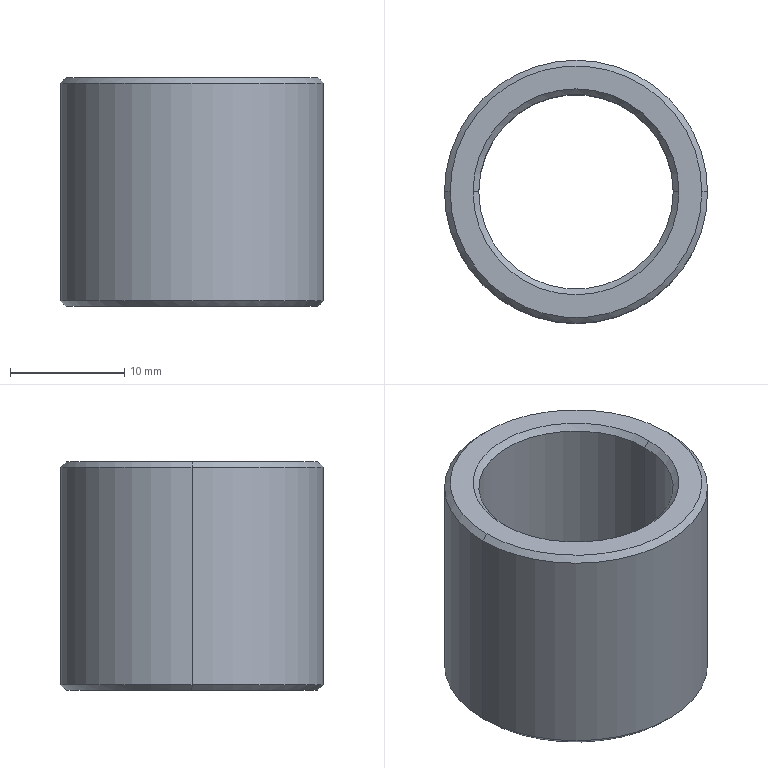Part | SolidWorks | features Chamfer 1, Extrusion 1 | 1 solid | 14 faces | box 23 x 23 x 20 mm | volume 3738 mm3 | cone 8 | cylinder 4 | plane 2 | commonest cylinder face diameters 17 x2 23 x2
STEP:
#1=CARTESIAN_POINT('',(-8.5,0.,19.5));
#2=VERTEX_POINT('',#1);
#3=CARTESIAN_POINT('',(8.5,0.,19.5));
#4=VERTEX_POINT('',#3);
#5=CARTESIAN_POINT('',(0.,0.,19.5));
#6=DIRECTION('',(0.,0.,1.));
#7=DIRECTION('',(1.,0.,0.));
#8=AXIS2_PLACEMENT_3D('',#5,#6,#7);
#9=CIRCLE('',#8,8.5);
#10=EDGE_CURVE('',#2,#4,#9,.T.);
#11=ORIENTED_EDGE('',*,*,#10,.F.);
#12=CARTESIAN_POINT('',(-9.,0.,20.));
#13=VERTEX_POINT('',#12);
#14=CARTESIAN_POINT('',(-8.5,0.,19.5));
#15=DIRECTION('',(-0.7071,0.,0.7071));
#16=VECTOR('',#15,1000.);
#17=LINE('',#14,#16);
#18=EDGE_CURVE('',#2,#13,#17,.T.);
#19=ORIENTED_EDGE('',*,*,#18,.T.);
#20=CARTESIAN_POINT('',(9.,0.,20.));
#21=VERTEX_POINT('',#20);
#22=CARTESIAN_POINT('',(0.,0.,20.));
#23=DIRECTION('',(0.,0.,-1.));
#24=DIRECTION('',(1.,0.,0.));
#25=AXIS2_PLACEMENT_3D('',#22,#23,#24);
#26=CIRCLE('',#25,9.);
#27=EDGE_CURVE('',#21,#13,#26,.T.);
#28=ORIENTED_EDGE('',*,*,#27,.F.);
#29=CARTESIAN_POINT('',(8.5,0.,19.5));
#30=DIRECTION('',(0.7071,0.,0.7071));
#31=VECTOR('',#30,1000.);
#32=LINE('',#29,#31);
#33=EDGE_CURVE('',#4,#21,#32,.T.);
#34=ORIENTED_EDGE('',*,*,#33,.F.);
#35=EDGE_LOOP('',(#11,#19,#28,#34));
#36=FACE_OUTER_BOUND('',#35,.T.);
#37=CARTESIAN_POINT('',(0.,0.,19.5));
#38=DIRECTION('',(0.,0.,1.));
#39=DIRECTION('',(1.,0.,0.));
#40=AXIS2_PLACEMENT_3D('',#37,#38,#39);
#41=CONICAL_SURFACE('',#40,8.5,0.7854);
#42=ADVANCED_FACE('',(#36),#41,.F.);
#43=CARTESIAN_POINT('',(11.,0.,20.));
#44=VERTEX_POINT('',#43);
#45=CARTESIAN_POINT('',(-11.,0.,20.));
#46=VERTEX_POINT('',#45);
#47=CARTESIAN_POINT('',(0.,0.,20.));
#48=DIRECTION('',(0.,0.,1.));
#49=DIRECTION('',(1.,0.,0.));
#50=AXIS2_PLACEMENT_3D('',#47,#48,#49);
#51=CIRCLE('',#50,11.);
#52=EDGE_CURVE('',#44,#46,#51,.T.);
#53=ORIENTED_EDGE('',*,*,#52,.F.);
#54=CARTESIAN_POINT('',(11.5,0.,19.5));
#55=VERTEX_POINT('',#54);
#56=CARTESIAN_POINT('',(11.,0.,20.));
#57=DIRECTION('',(0.7071,0.,-0.7071));
#58=VECTOR('',#57,1000.);
#59=LINE('',#56,#58);
#60=EDGE_CURVE('',#44,#55,#59,.T.);
#61=ORIENTED_EDGE('',*,*,#60,.T.);
#62=CARTESIAN_POINT('',(-11.5,0.,19.5));
#63=VERTEX_POINT('',#62);
#64=CARTESIAN_POINT('',(0.,0.,19.5));
#65=DIRECTION('',(0.,0.,-1.));
#66=DIRECTION('',(1.,0.,0.));
#67=AXIS2_PLACEMENT_3D('',#64,#65,#66);
#68=CIRCLE('',#67,11.5);
#69=EDGE_CURVE('',#63,#55,#68,.T.);
#70=ORIENTED_EDGE('',*,*,#69,.F.);
#71=CARTESIAN_POINT('',(-11.,0.,20.));
#72=DIRECTION('',(-0.7071,0.,-0.7071));
#73=VECTOR('',#72,1000.);
#74=LINE('',#71,#73);
#75=EDGE_CURVE('',#46,#63,#74,.T.);
#76=ORIENTED_EDGE('',*,*,#75,.F.);
#77=EDGE_LOOP('',(#53,#61,#70,#76));
#78=FACE_OUTER_BOUND('',#77,.T.);
#79=CARTESIAN_POINT('',(0.,0.,20.));
#80=DIRECTION('',(0.,0.,-1.));
#81=DIRECTION('',(-1.,0.,0.));
#82=AXIS2_PLACEMENT_3D('',#79,#80,#81);
#83=CONICAL_SURFACE('',#82,11.,0.7854);
#84=ADVANCED_FACE('',(#78),#83,.T.);
#85=CARTESIAN_POINT('',(8.5,0.,0.5));
#86=VERTEX_POINT('',#85);
#87=CARTESIAN_POINT('',(-8.5,0.,0.5));
#88=VERTEX_POINT('',#87);
#89=CARTESIAN_POINT('',(0.,0.,0.5));
#90=DIRECTION('',(0.,0.,-1.));
#91=DIRECTION('',(1.,0.,0.));
#92=AXIS2_PLACEMENT_3D('',#89,#90,#91);
#93=CIRCLE('',#92,8.5);
#94=EDGE_CURVE('',#86,#88,#93,.T.);
#95=ORIENTED_EDGE('',*,*,#94,.F.);
#96=CARTESIAN_POINT('',(9.,0.,0.));
#97=VERTEX_POINT('',#96);
#98=CARTESIAN_POINT('',(9.,0.,0.));
#99=DIRECTION('',(0.7071,0.,-0.7071));
#100=VECTOR('',#99,1000.);
#101=LINE('',#98,#100);
#102=EDGE_CURVE('',#86,#97,#101,.T.);
#103=ORIENTED_EDGE('',*,*,#102,.T.);
#104=CARTESIAN_POINT('',(-9.,0.,0.));
#105=VERTEX_POINT('',#104);
#106=CARTESIAN_POINT('',(0.,0.,0.));
#107=DIRECTION('',(0.,0.,1.));
#108=DIRECTION('',(1.,0.,0.));
#109=AXIS2_PLACEMENT_3D('',#106,#107,#108);
#110=CIRCLE('',#109,9.);
#111=EDGE_CURVE('',#105,#97,#110,.T.);
#112=ORIENTED_EDGE('',*,*,#111,.F.);
#113=CARTESIAN_POINT('',(-9.,0.,0.));
#114=DIRECTION('',(-0.7071,0.,-0.7071));
#115=VECTOR('',#114,1000.);
#116=LINE('',#113,#115);
#117=EDGE_CURVE('',#88,#105,#116,.T.);
#118=ORIENTED_EDGE('',*,*,#117,.F.);
#119=EDGE_LOOP('',(#95,#103,#112,#118));
#120=FACE_OUTER_BOUND('',#119,.T.);
#121=CARTESIAN_POINT('',(0.,0.,0.));
#122=DIRECTION('',(0.,0.,-1.));
#123=DIRECTION('',(-1.,0.,0.));
#124=AXIS2_PLACEMENT_3D('',#121,#122,#123);
#125=CONICAL_SURFACE('',#124,9.,0.7854);
#126=ADVANCED_FACE('',(#120),#125,.F.);
#127=CARTESIAN_POINT('',(-11.,0.,0.));
#128=VERTEX_POINT('',#127);
#129=CARTESIAN_POINT('',(11.,0.,0.));
#130=VERTEX_POINT('',#129);
#131=CARTESIAN_POINT('',(0.,0.,0.));
#132=DIRECTION('',(0.,0.,-1.));
#133=DIRECTION('',(1.,0.,0.));
#134=AXIS2_PLACEMENT_3D('',#131,#132,#133);
#135=CIRCLE('',#134,11.);
#136=EDGE_CURVE('',#128,#130,#135,.T.);
#137=ORIENTED_EDGE('',*,*,#136,.F.);
#138=CARTESIAN_POINT('',(-11.5,0.,0.5));
#139=VERTEX_POINT('',#138);
#140=CARTESIAN_POINT('',(-11.5,0.,0.5));
#141=DIRECTION('',(-0.7071,0.,0.7071));
#142=VECTOR('',#141,1000.);
#143=LINE('',#140,#142);
#144=EDGE_CURVE('',#128,#139,#143,.T.);
#145=ORIENTED_EDGE('',*,*,#144,.T.);
#146=CARTESIAN_POINT('',(11.5,0.,0.5));
#147=VERTEX_POINT('',#146);
#148=CARTESIAN_POINT('',(0.,0.,0.5));
#149=DIRECTION('',(0.,0.,1.));
#150=DIRECTION('',(1.,0.,0.));
#151=AXIS2_PLACEMENT_3D('',#148,#149,#150);
#152=CIRCLE('',#151,11.5);
#153=EDGE_CURVE('',#147,#139,#152,.T.);
#154=ORIENTED_EDGE('',*,*,#153,.F.);
#155=CARTESIAN_POINT('',(11.5,0.,0.5));
#156=DIRECTION('',(0.7071,0.,0.7071));
#157=VECTOR('',#156,1000.);
#158=LINE('',#155,#157);
#159=EDGE_CURVE('',#130,#147,#158,.T.);
#160=ORIENTED_EDGE('',*,*,#159,.F.);
#161=EDGE_LOOP('',(#137,#145,#154,#160));
#162=FACE_OUTER_BOUND('',#161,.T.);
#163=CARTESIAN_POINT('',(0.,0.,0.5));
#164=DIRECTION('',(0.,0.,1.));
#165=DIRECTION('',(1.,0.,0.));
#166=AXIS2_PLACEMENT_3D('',#163,#164,#165);
#167=CONICAL_SURFACE('',#166,11.5,0.7854);
#168=ADVANCED_FACE('',(#162),#167,.T.);
#169=ORIENTED_EDGE('',*,*,#10,.T.);
#170=CARTESIAN_POINT('',(8.5,0.,20.));
#171=DIRECTION('',(0.,0.,-1.));
#172=VECTOR('',#171,1000.);
#173=LINE('',#170,#172);
#174=EDGE_CURVE('',#4,#86,#173,.T.);
#175=ORIENTED_EDGE('',*,*,#174,.T.);
#176=ORIENTED_EDGE('',*,*,#94,.T.);
#177=CARTESIAN_POINT('',(-8.5,0.,20.));
#178=DIRECTION('',(0.,0.,-1.));
#179=VECTOR('',#178,1000.);
#180=LINE('',#177,#179);
#181=EDGE_CURVE('',#2,#88,#180,.T.);
#182=ORIENTED_EDGE('',*,*,#181,.F.);
#183=EDGE_LOOP('',(#169,#175,#176,#182));
#184=FACE_OUTER_BOUND('',#183,.T.);
#185=CARTESIAN_POINT('',(0.,0.,20.));
#186=DIRECTION('',(0.,0.,-1.));
#187=DIRECTION('',(-1.,0.,0.));
#188=AXIS2_PLACEMENT_3D('',#185,#186,#187);
#189=CYLINDRICAL_SURFACE('',#188,8.5);
#190=ADVANCED_FACE('',(#184),#189,.F.);
#191=ORIENTED_EDGE('',*,*,#69,.T.);
#192=CARTESIAN_POINT('',(11.5,0.,20.));
#193=DIRECTION('',(0.,0.,-1.));
#194=VECTOR('',#193,1000.);
#195=LINE('',#192,#194);
#196=EDGE_CURVE('',#55,#147,#195,.T.);
#197=ORIENTED_EDGE('',*,*,#196,.T.);
#198=ORIENTED_EDGE('',*,*,#153,.T.);
#199=CARTESIAN_POINT('',(-11.5,0.,20.));
#200=DIRECTION('',(0.,0.,-1.));
#201=VECTOR('',#200,1000.);
#202=LINE('',#199,#201);
#203=EDGE_CURVE('',#63,#139,#202,.T.);
#204=ORIENTED_EDGE('',*,*,#203,.F.);
#205=EDGE_LOOP('',(#191,#197,#198,#204));
#206=FACE_OUTER_BOUND('',#205,.T.);
#207=CARTESIAN_POINT('',(0.,0.,20.));
#208=DIRECTION('',(0.,0.,-1.));
#209=DIRECTION('',(-1.,0.,0.));
#210=AXIS2_PLACEMENT_3D('',#207,#208,#209);
#211=CYLINDRICAL_SURFACE('',#210,11.5);
#212=ADVANCED_FACE('',(#206),#211,.T.);
#213=CARTESIAN_POINT('',(0.,0.,20.));
#214=DIRECTION('',(0.,0.,1.));
#215=DIRECTION('',(1.,0.,0.));
#216=AXIS2_PLACEMENT_3D('',#213,#214,#215);
#217=CIRCLE('',#216,11.);
#218=EDGE_CURVE('',#46,#44,#217,.T.);
#219=ORIENTED_EDGE('',*,*,#218,.T.);
#220=ORIENTED_EDGE('',*,*,#52,.T.);
#221=EDGE_LOOP('',(#219,#220));
#222=FACE_OUTER_BOUND('',#221,.T.);
#223=ORIENTED_EDGE('',*,*,#27,.T.);
#224=CARTESIAN_POINT('',(0.,0.,20.));
#225=DIRECTION('',(0.,0.,-1.));
#226=DIRECTION('',(1.,0.,0.));
#227=AXIS2_PLACEMENT_3D('',#224,#225,#226);
#228=CIRCLE('',#227,9.);
#229=EDGE_CURVE('',#13,#21,#228,.T.);
#230=ORIENTED_EDGE('',*,*,#229,.T.);
#231=EDGE_LOOP('',(#223,#230));
#232=FACE_BOUND('',#231,.T.);
#233=CARTESIAN_POINT('',(0.,0.,20.));
#234=DIRECTION('',(0.,0.,1.));
#235=DIRECTION('',(1.,0.,0.));
#236=AXIS2_PLACEMENT_3D('',#233,#234,#235);
#237=PLANE('',#236);
#238=ADVANCED_FACE('',(#222,#232),#237,.T.);
#239=CARTESIAN_POINT('',(0.,0.,0.));
#240=DIRECTION('',(0.,0.,-1.));
#241=DIRECTION('',(1.,0.,0.));
#242=AXIS2_PLACEMENT_3D('',#239,#240,#241);
#243=CIRCLE('',#242,11.);
#244=EDGE_CURVE('',#130,#128,#243,.T.);
#245=ORIENTED_EDGE('',*,*,#244,.T.);
#246=ORIENTED_EDGE('',*,*,#136,.T.);
#247=EDGE_LOOP('',(#245,#246));
#248=FACE_OUTER_BOUND('',#247,.T.);
#249=ORIENTED_EDGE('',*,*,#111,.T.);
#250=CARTESIAN_POINT('',(0.,0.,0.));
#251=DIRECTION('',(0.,0.,1.));
#252=DIRECTION('',(1.,0.,0.));
#253=AXIS2_PLACEMENT_3D('',#250,#251,#252);
#254=CIRCLE('',#253,9.);
#255=EDGE_CURVE('',#97,#105,#254,.T.);
#256=ORIENTED_EDGE('',*,*,#255,.T.);
#257=EDGE_LOOP('',(#249,#256));
#258=FACE_BOUND('',#257,.T.);
#259=CARTESIAN_POINT('',(0.,0.,0.));
#260=DIRECTION('',(0.,0.,1.));
#261=DIRECTION('',(1.,0.,0.));
#262=AXIS2_PLACEMENT_3D('',#259,#260,#261);
#263=PLANE('',#262);
#264=ADVANCED_FACE('',(#248,#258),#263,.F.);
#265=ORIENTED_EDGE('',*,*,#196,.F.);
#266=CARTESIAN_POINT('',(0.,0.,19.5));
#267=DIRECTION('',(0.,0.,-1.));
#268=DIRECTION('',(1.,0.,0.));
#269=AXIS2_PLACEMENT_3D('',#266,#267,#268);
#270=CIRCLE('',#269,11.5);
#271=EDGE_CURVE('',#55,#63,#270,.T.);
#272=ORIENTED_EDGE('',*,*,#271,.T.);
#273=ORIENTED_EDGE('',*,*,#203,.T.);
#274=CARTESIAN_POINT('',(0.,0.,0.5));
#275=DIRECTION('',(0.,0.,1.));
#276=DIRECTION('',(1.,0.,0.));
#277=AXIS2_PLACEMENT_3D('',#274,#275,#276);
#278=CIRCLE('',#277,11.5);
#279=EDGE_CURVE('',#139,#147,#278,.T.);
#280=ORIENTED_EDGE('',*,*,#279,.T.);
#281=EDGE_LOOP('',(#265,#272,#273,#280));
#282=FACE_OUTER_BOUND('',#281,.T.);
#283=CARTESIAN_POINT('',(0.,0.,20.));
#284=DIRECTION('',(0.,0.,-1.));
#285=DIRECTION('',(-1.,0.,0.));
#286=AXIS2_PLACEMENT_3D('',#283,#284,#285);
#287=CYLINDRICAL_SURFACE('',#286,11.5);
#288=ADVANCED_FACE('',(#282),#287,.T.);
#289=ORIENTED_EDGE('',*,*,#174,.F.);
#290=CARTESIAN_POINT('',(0.,0.,19.5));
#291=DIRECTION('',(0.,0.,1.));
#292=DIRECTION('',(1.,0.,0.));
#293=AXIS2_PLACEMENT_3D('',#290,#291,#292);
#294=CIRCLE('',#293,8.5);
#295=EDGE_CURVE('',#4,#2,#294,.T.);
#296=ORIENTED_EDGE('',*,*,#295,.T.);
#297=ORIENTED_EDGE('',*,*,#181,.T.);
#298=CARTESIAN_POINT('',(0.,0.,0.5));
#299=DIRECTION('',(0.,0.,-1.));
#300=DIRECTION('',(1.,0.,0.));
#301=AXIS2_PLACEMENT_3D('',#298,#299,#300);
#302=CIRCLE('',#301,8.5);
#303=EDGE_CURVE('',#88,#86,#302,.T.);
#304=ORIENTED_EDGE('',*,*,#303,.T.);
#305=EDGE_LOOP('',(#289,#296,#297,#304));
#306=FACE_OUTER_BOUND('',#305,.T.);
#307=CARTESIAN_POINT('',(0.,0.,20.));
#308=DIRECTION('',(0.,0.,-1.));
#309=DIRECTION('',(-1.,0.,0.));
#310=AXIS2_PLACEMENT_3D('',#307,#308,#309);
#311=CYLINDRICAL_SURFACE('',#310,8.5);
#312=ADVANCED_FACE('',(#306),#311,.F.);
#313=ORIENTED_EDGE('',*,*,#144,.F.);
#314=ORIENTED_EDGE('',*,*,#244,.F.);
#315=ORIENTED_EDGE('',*,*,#159,.T.);
#316=ORIENTED_EDGE('',*,*,#279,.F.);
#317=EDGE_LOOP('',(#313,#314,#315,#316));
#318=FACE_OUTER_BOUND('',#317,.T.);
#319=CARTESIAN_POINT('',(0.,0.,0.5));
#320=DIRECTION('',(0.,0.,1.));
#321=DIRECTION('',(1.,0.,0.));
#322=AXIS2_PLACEMENT_3D('',#319,#320,#321);
#323=CONICAL_SURFACE('',#322,11.5,0.7854);
#324=ADVANCED_FACE('',(#318),#323,.T.);
#325=ORIENTED_EDGE('',*,*,#102,.F.);
#326=ORIENTED_EDGE('',*,*,#303,.F.);
#327=ORIENTED_EDGE('',*,*,#117,.T.);
#328=ORIENTED_EDGE('',*,*,#255,.F.);
#329=EDGE_LOOP('',(#325,#326,#327,#328));
#330=FACE_OUTER_BOUND('',#329,.T.);
#331=CARTESIAN_POINT('',(0.,0.,0.));
#332=DIRECTION('',(0.,0.,-1.));
#333=DIRECTION('',(-1.,0.,0.));
#334=AXIS2_PLACEMENT_3D('',#331,#332,#333);
#335=CONICAL_SURFACE('',#334,9.,0.7854);
#336=ADVANCED_FACE('',(#330),#335,.F.);
#337=ORIENTED_EDGE('',*,*,#60,.F.);
#338=ORIENTED_EDGE('',*,*,#218,.F.);
#339=ORIENTED_EDGE('',*,*,#75,.T.);
#340=ORIENTED_EDGE('',*,*,#271,.F.);
#341=EDGE_LOOP('',(#337,#338,#339,#340));
#342=FACE_OUTER_BOUND('',#341,.T.);
#343=CARTESIAN_POINT('',(0.,0.,20.));
#344=DIRECTION('',(0.,0.,-1.));
#345=DIRECTION('',(-1.,0.,0.));
#346=AXIS2_PLACEMENT_3D('',#343,#344,#345);
#347=CONICAL_SURFACE('',#346,11.,0.7854);
#348=ADVANCED_FACE('',(#342),#347,.T.);
#349=ORIENTED_EDGE('',*,*,#18,.F.);
#350=ORIENTED_EDGE('',*,*,#295,.F.);
#351=ORIENTED_EDGE('',*,*,#33,.T.);
#352=ORIENTED_EDGE('',*,*,#229,.F.);
#353=EDGE_LOOP('',(#349,#350,#351,#352));
#354=FACE_OUTER_BOUND('',#353,.T.);
#355=CARTESIAN_POINT('',(0.,0.,19.5));
#356=DIRECTION('',(0.,0.,1.));
#357=DIRECTION('',(1.,0.,0.));
#358=AXIS2_PLACEMENT_3D('',#355,#356,#357);
#359=CONICAL_SURFACE('',#358,8.5,0.7854);
#360=ADVANCED_FACE('',(#354),#359,.F.);
#361=CLOSED_SHELL('',(#42,#84,#126,#168,#190,#212,#238,#264,#288,#312,#324,#336,#348,#360));
#362=MANIFOLD_SOLID_BREP('',#361);
#363=CARTESIAN_POINT('',(0.,0.,0.));
#364=DIRECTION('',(0.,0.,1.));
#365=DIRECTION('',(1.,0.,0.));
#366=AXIS2_PLACEMENT_3D('',#363,#364,#365);
#367=(LENGTH_UNIT()NAMED_UNIT(*)SI_UNIT(.MILLI.,.METRE.));
#368=UNCERTAINTY_MEASURE_WITH_UNIT(LENGTH_MEASURE(0.00001),#367,'','');
#369=(NAMED_UNIT(*)PLANE_ANGLE_UNIT()SI_UNIT($,.RADIAN.));
#370=(NAMED_UNIT(*)SI_UNIT($,.STERADIAN.)SOLID_ANGLE_UNIT());
#371=(GEOMETRIC_REPRESENTATION_CONTEXT(3)GLOBAL_UNCERTAINTY_ASSIGNED_CONTEXT((#368))GLOBAL_UNIT_ASSIGNED_CONTEXT((#367,#369,#370))REPRESENTATION_CONTEXT('',''));
#372=ADVANCED_BREP_SHAPE_REPRESENTATION('',(#362,#366),#371);